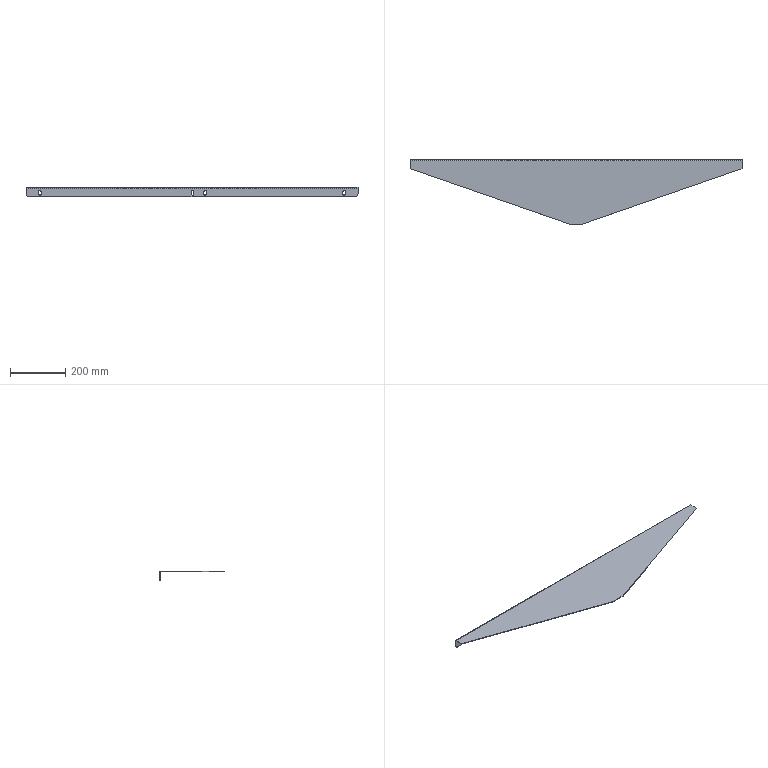Part | SolidWorks | features MirrorStock 1 | 1 solid | 38 faces | box 1200 x 232 x 34 mm | volume 400369 mm3 | plane 22 | cylinder 16 | commonest cylinder face diameters 9 x12 20 x2 2 x1 6 x1
STEP:
#1=CARTESIAN_POINT('',(45.5,0.,-26.));
#2=VERTEX_POINT('',#1);
#3=CARTESIAN_POINT('',(50.,0.,-30.5));
#4=VERTEX_POINT('',#3);
#5=CARTESIAN_POINT('',(50.,0.,-26.));
#6=DIRECTION('',(0.,-1.,0.));
#7=DIRECTION('',(0.,0.,-1.));
#8=AXIS2_PLACEMENT_3D('',#5,#6,#7);
#9=CIRCLE('',#8,4.5);
#10=EDGE_CURVE('',#2,#4,#9,.T.);
#11=ORIENTED_EDGE('',*,*,#10,.T.);
#12=CARTESIAN_POINT('',(50.,2.,-30.5));
#13=VERTEX_POINT('',#12);
#14=CARTESIAN_POINT('',(50.,-8.,-30.5));
#15=DIRECTION('',(0.,1.,0.));
#16=VECTOR('',#15,1000.);
#17=LINE('',#14,#16);
#18=EDGE_CURVE('',#4,#13,#17,.T.);
#19=ORIENTED_EDGE('',*,*,#18,.T.);
#20=CARTESIAN_POINT('',(45.5,2.,-26.));
#21=VERTEX_POINT('',#20);
#22=CARTESIAN_POINT('',(50.,2.,-26.));
#23=DIRECTION('',(0.,-1.,0.));
#24=DIRECTION('',(0.,0.,-1.));
#25=AXIS2_PLACEMENT_3D('',#22,#23,#24);
#26=CIRCLE('',#25,4.5);
#27=EDGE_CURVE('',#21,#13,#26,.T.);
#28=ORIENTED_EDGE('',*,*,#27,.F.);
#29=CARTESIAN_POINT('',(45.5,-8.,-26.));
#30=DIRECTION('',(0.,1.,0.));
#31=VECTOR('',#30,1000.);
#32=LINE('',#29,#31);
#33=EDGE_CURVE('',#2,#21,#32,.T.);
#34=ORIENTED_EDGE('',*,*,#33,.F.);
#35=EDGE_LOOP('',(#11,#19,#28,#34));
#36=FACE_OUTER_BOUND('',#35,.T.);
#37=CARTESIAN_POINT('',(50.,-8.,-26.));
#38=DIRECTION('',(0.,1.,0.));
#39=DIRECTION('',(0.,0.,-1.));
#40=AXIS2_PLACEMENT_3D('',#37,#38,#39);
#41=CYLINDRICAL_SURFACE('',#40,4.5);
#42=ADVANCED_FACE('',(#36),#41,.F.);
#43=CARTESIAN_POINT('',(1145.5,0.,-26.));
#44=VERTEX_POINT('',#43);
#45=CARTESIAN_POINT('',(1150.,0.,-30.5));
#46=VERTEX_POINT('',#45);
#47=CARTESIAN_POINT('',(1150.,0.,-26.));
#48=DIRECTION('',(0.,-1.,0.));
#49=DIRECTION('',(0.,0.,-1.));
#50=AXIS2_PLACEMENT_3D('',#47,#48,#49);
#51=CIRCLE('',#50,4.5);
#52=EDGE_CURVE('',#44,#46,#51,.T.);
#53=ORIENTED_EDGE('',*,*,#52,.T.);
#54=CARTESIAN_POINT('',(1150.,2.,-30.5));
#55=VERTEX_POINT('',#54);
#56=CARTESIAN_POINT('',(1150.,-8.,-30.5));
#57=DIRECTION('',(0.,1.,0.));
#58=VECTOR('',#57,1000.);
#59=LINE('',#56,#58);
#60=EDGE_CURVE('',#46,#55,#59,.T.);
#61=ORIENTED_EDGE('',*,*,#60,.T.);
#62=CARTESIAN_POINT('',(1145.5,2.,-26.));
#63=VERTEX_POINT('',#62);
#64=CARTESIAN_POINT('',(1150.,2.,-26.));
#65=DIRECTION('',(0.,-1.,0.));
#66=DIRECTION('',(0.,0.,-1.));
#67=AXIS2_PLACEMENT_3D('',#64,#65,#66);
#68=CIRCLE('',#67,4.5);
#69=EDGE_CURVE('',#63,#55,#68,.T.);
#70=ORIENTED_EDGE('',*,*,#69,.F.);
#71=CARTESIAN_POINT('',(1145.5,-8.,-26.));
#72=DIRECTION('',(0.,1.,0.));
#73=VECTOR('',#72,1000.);
#74=LINE('',#71,#73);
#75=EDGE_CURVE('',#44,#63,#74,.T.);
#76=ORIENTED_EDGE('',*,*,#75,.F.);
#77=EDGE_LOOP('',(#53,#61,#70,#76));
#78=FACE_OUTER_BOUND('',#77,.T.);
#79=CARTESIAN_POINT('',(1150.,-8.,-26.));
#80=DIRECTION('',(0.,1.,0.));
#81=DIRECTION('',(0.,0.,-1.));
#82=AXIS2_PLACEMENT_3D('',#79,#80,#81);
#83=CYLINDRICAL_SURFACE('',#82,4.5);
#84=ADVANCED_FACE('',(#78),#83,.F.);
#85=CARTESIAN_POINT('',(598.,0.,-26.));
#86=VERTEX_POINT('',#85);
#87=CARTESIAN_POINT('',(602.5,0.,-30.5));
#88=VERTEX_POINT('',#87);
#89=CARTESIAN_POINT('',(602.5,0.,-26.));
#90=DIRECTION('',(0.,-1.,0.));
#91=DIRECTION('',(0.,0.,-1.));
#92=AXIS2_PLACEMENT_3D('',#89,#90,#91);
#93=CIRCLE('',#92,4.5);
#94=EDGE_CURVE('',#86,#88,#93,.T.);
#95=ORIENTED_EDGE('',*,*,#94,.T.);
#96=CARTESIAN_POINT('',(602.5,2.,-30.5));
#97=VERTEX_POINT('',#96);
#98=CARTESIAN_POINT('',(602.5,-8.,-30.5));
#99=DIRECTION('',(0.,1.,0.));
#100=VECTOR('',#99,1000.);
#101=LINE('',#98,#100);
#102=EDGE_CURVE('',#88,#97,#101,.T.);
#103=ORIENTED_EDGE('',*,*,#102,.T.);
#104=CARTESIAN_POINT('',(598.,2.,-26.));
#105=VERTEX_POINT('',#104);
#106=CARTESIAN_POINT('',(602.5,2.,-26.));
#107=DIRECTION('',(0.,-1.,0.));
#108=DIRECTION('',(0.,0.,-1.));
#109=AXIS2_PLACEMENT_3D('',#106,#107,#108);
#110=CIRCLE('',#109,4.5);
#111=EDGE_CURVE('',#105,#97,#110,.T.);
#112=ORIENTED_EDGE('',*,*,#111,.F.);
#113=CARTESIAN_POINT('',(598.,-8.,-26.));
#114=DIRECTION('',(0.,1.,0.));
#115=VECTOR('',#114,1000.);
#116=LINE('',#113,#115);
#117=EDGE_CURVE('',#86,#105,#116,.T.);
#118=ORIENTED_EDGE('',*,*,#117,.F.);
#119=EDGE_LOOP('',(#95,#103,#112,#118));
#120=FACE_OUTER_BOUND('',#119,.T.);
#121=CARTESIAN_POINT('',(602.5,-8.,-26.));
#122=DIRECTION('',(0.,1.,0.));
#123=DIRECTION('',(0.,0.,-1.));
#124=AXIS2_PLACEMENT_3D('',#121,#122,#123);
#125=CYLINDRICAL_SURFACE('',#124,4.5);
#126=ADVANCED_FACE('',(#120),#125,.F.);
#127=CARTESIAN_POINT('',(643.,0.,-26.));
#128=VERTEX_POINT('',#127);
#129=CARTESIAN_POINT('',(647.5,0.,-30.5));
#130=VERTEX_POINT('',#129);
#131=CARTESIAN_POINT('',(647.5,0.,-26.));
#132=DIRECTION('',(0.,-1.,0.));
#133=DIRECTION('',(0.,0.,-1.));
#134=AXIS2_PLACEMENT_3D('',#131,#132,#133);
#135=CIRCLE('',#134,4.5);
#136=EDGE_CURVE('',#128,#130,#135,.T.);
#137=ORIENTED_EDGE('',*,*,#136,.T.);
#138=CARTESIAN_POINT('',(647.5,2.,-30.5));
#139=VERTEX_POINT('',#138);
#140=CARTESIAN_POINT('',(647.5,-8.,-30.5));
#141=DIRECTION('',(0.,1.,0.));
#142=VECTOR('',#141,1000.);
#143=LINE('',#140,#142);
#144=EDGE_CURVE('',#130,#139,#143,.T.);
#145=ORIENTED_EDGE('',*,*,#144,.T.);
#146=CARTESIAN_POINT('',(643.,2.,-26.));
#147=VERTEX_POINT('',#146);
#148=CARTESIAN_POINT('',(647.5,2.,-26.));
#149=DIRECTION('',(0.,-1.,0.));
#150=DIRECTION('',(0.,0.,1.));
#151=AXIS2_PLACEMENT_3D('',#148,#149,#150);
#152=CIRCLE('',#151,4.5);
#153=EDGE_CURVE('',#147,#139,#152,.T.);
#154=ORIENTED_EDGE('',*,*,#153,.F.);
#155=CARTESIAN_POINT('',(643.,-8.,-26.));
#156=DIRECTION('',(0.,1.,0.));
#157=VECTOR('',#156,1000.);
#158=LINE('',#155,#157);
#159=EDGE_CURVE('',#128,#147,#158,.T.);
#160=ORIENTED_EDGE('',*,*,#159,.F.);
#161=EDGE_LOOP('',(#137,#145,#154,#160));
#162=FACE_OUTER_BOUND('',#161,.T.);
#163=CARTESIAN_POINT('',(647.5,-8.,-26.));
#164=DIRECTION('',(0.,1.,0.));
#165=DIRECTION('',(0.,0.,-1.));
#166=AXIS2_PLACEMENT_3D('',#163,#164,#165);
#167=CYLINDRICAL_SURFACE('',#166,4.5);
#168=ADVANCED_FACE('',(#162),#167,.F.);
#169=CARTESIAN_POINT('',(0.,-1.,-4.));
#170=VERTEX_POINT('',#169);
#171=CARTESIAN_POINT('',(0.,-30.,-4.));
#172=VERTEX_POINT('',#171);
#173=CARTESIAN_POINT('',(0.,0.,-4.));
#174=DIRECTION('',(0.,-1.,0.));
#175=VECTOR('',#174,1000.);
#176=LINE('',#173,#175);
#177=EDGE_CURVE('',#170,#172,#176,.T.);
#178=ORIENTED_EDGE('',*,*,#177,.T.);
#179=CARTESIAN_POINT('',(0.,-30.,-2.));
#180=VERTEX_POINT('',#179);
#181=CARTESIAN_POINT('',(0.,-30.,-2.));
#182=DIRECTION('',(0.,0.,-1.));
#183=VECTOR('',#182,1000.);
#184=LINE('',#181,#183);
#185=EDGE_CURVE('',#180,#172,#184,.T.);
#186=ORIENTED_EDGE('',*,*,#185,.F.);
#187=CARTESIAN_POINT('',(0.,-1.,-2.));
#188=VERTEX_POINT('',#187);
#189=CARTESIAN_POINT('',(0.,0.,-2.));
#190=DIRECTION('',(0.,-1.,0.));
#191=VECTOR('',#190,1000.);
#192=LINE('',#189,#191);
#193=EDGE_CURVE('',#188,#180,#192,.T.);
#194=ORIENTED_EDGE('',*,*,#193,.F.);
#195=CARTESIAN_POINT('',(0.,-1.,-4.));
#196=DIRECTION('',(0.,0.,1.));
#197=VECTOR('',#196,1000.);
#198=LINE('',#195,#197);
#199=EDGE_CURVE('',#170,#188,#198,.T.);
#200=ORIENTED_EDGE('',*,*,#199,.F.);
#201=EDGE_LOOP('',(#178,#186,#194,#200));
#202=FACE_OUTER_BOUND('',#201,.T.);
#203=CARTESIAN_POINT('',(0.,0.,-2.));
#204=DIRECTION('',(-1.,0.,0.));
#205=DIRECTION('',(0.,-1.,0.));
#206=AXIS2_PLACEMENT_3D('',#203,#204,#205);
#207=PLANE('',#206);
#208=ADVANCED_FACE('',(#202),#207,.T.);
#209=ORIENTED_EDGE('',*,*,#193,.T.);
#210=CARTESIAN_POINT('',(575.,-230.,-2.));
#211=VERTEX_POINT('',#210);
#212=CARTESIAN_POINT('',(0.,-30.,-2.));
#213=DIRECTION('',(0.9445,-0.3285,0.));
#214=VECTOR('',#213,1000.);
#215=LINE('',#212,#214);
#216=EDGE_CURVE('',#180,#211,#215,.T.);
#217=ORIENTED_EDGE('',*,*,#216,.T.);
#218=CARTESIAN_POINT('',(625.,-230.,-2.));
#219=VERTEX_POINT('',#218);
#220=CARTESIAN_POINT('',(625.,-230.,-2.));
#221=DIRECTION('',(1.,0.,0.));
#222=VECTOR('',#221,1000.);
#223=LINE('',#220,#222);
#224=EDGE_CURVE('',#211,#219,#223,.T.);
#225=ORIENTED_EDGE('',*,*,#224,.T.);
#226=CARTESIAN_POINT('',(1200.,-30.,-2.));
#227=VERTEX_POINT('',#226);
#228=CARTESIAN_POINT('',(1200.,-30.,-2.));
#229=DIRECTION('',(0.9445,0.3285,0.));
#230=VECTOR('',#229,1000.);
#231=LINE('',#228,#230);
#232=EDGE_CURVE('',#219,#227,#231,.T.);
#233=ORIENTED_EDGE('',*,*,#232,.T.);
#234=CARTESIAN_POINT('',(1200.,-1.,-2.));
#235=VERTEX_POINT('',#234);
#236=CARTESIAN_POINT('',(1200.,0.,-2.));
#237=DIRECTION('',(0.,1.,0.));
#238=VECTOR('',#237,1000.);
#239=LINE('',#236,#238);
#240=EDGE_CURVE('',#227,#235,#239,.T.);
#241=ORIENTED_EDGE('',*,*,#240,.T.);
#242=CARTESIAN_POINT('',(0.,-1.,-2.));
#243=DIRECTION('',(1.,0.,0.));
#244=VECTOR('',#243,1000.);
#245=LINE('',#242,#244);
#246=EDGE_CURVE('',#188,#235,#245,.T.);
#247=ORIENTED_EDGE('',*,*,#246,.F.);
#248=EDGE_LOOP('',(#209,#217,#225,#233,#241,#247));
#249=FACE_OUTER_BOUND('',#248,.T.);
#250=CARTESIAN_POINT('',(0.,0.,-2.));
#251=DIRECTION('',(0.,0.,1.));
#252=DIRECTION('',(-1.,0.,0.));
#253=AXIS2_PLACEMENT_3D('',#250,#251,#252);
#254=PLANE('',#253);
#255=ADVANCED_FACE('',(#249),#254,.T.);
#256=CARTESIAN_POINT('',(1200.,-1.,-4.));
#257=VERTEX_POINT('',#256);
#258=CARTESIAN_POINT('',(0.,-1.,-4.));
#259=DIRECTION('',(1.,0.,0.));
#260=VECTOR('',#259,1000.);
#261=LINE('',#258,#260);
#262=EDGE_CURVE('',#170,#257,#261,.T.);
#263=ORIENTED_EDGE('',*,*,#262,.T.);
#264=CARTESIAN_POINT('',(1200.,-30.,-4.));
#265=VERTEX_POINT('',#264);
#266=CARTESIAN_POINT('',(1200.,0.,-4.));
#267=DIRECTION('',(0.,1.,0.));
#268=VECTOR('',#267,1000.);
#269=LINE('',#266,#268);
#270=EDGE_CURVE('',#265,#257,#269,.T.);
#271=ORIENTED_EDGE('',*,*,#270,.F.);
#272=CARTESIAN_POINT('',(625.,-230.,-4.));
#273=VERTEX_POINT('',#272);
#274=CARTESIAN_POINT('',(1200.,-30.,-4.));
#275=DIRECTION('',(0.9445,0.3285,0.));
#276=VECTOR('',#275,1000.);
#277=LINE('',#274,#276);
#278=EDGE_CURVE('',#273,#265,#277,.T.);
#279=ORIENTED_EDGE('',*,*,#278,.F.);
#280=CARTESIAN_POINT('',(575.,-230.,-4.));
#281=VERTEX_POINT('',#280);
#282=CARTESIAN_POINT('',(625.,-230.,-4.));
#283=DIRECTION('',(1.,0.,0.));
#284=VECTOR('',#283,1000.);
#285=LINE('',#282,#284);
#286=EDGE_CURVE('',#281,#273,#285,.T.);
#287=ORIENTED_EDGE('',*,*,#286,.F.);
#288=CARTESIAN_POINT('',(0.,-30.,-4.));
#289=DIRECTION('',(0.9445,-0.3285,0.));
#290=VECTOR('',#289,1000.);
#291=LINE('',#288,#290);
#292=EDGE_CURVE('',#172,#281,#291,.T.);
#293=ORIENTED_EDGE('',*,*,#292,.F.);
#294=ORIENTED_EDGE('',*,*,#177,.F.);
#295=EDGE_LOOP('',(#263,#271,#279,#287,#293,#294));
#296=FACE_OUTER_BOUND('',#295,.T.);
#297=CARTESIAN_POINT('',(0.,0.,-4.));
#298=DIRECTION('',(0.,0.,1.));
#299=DIRECTION('',(-1.,0.,0.));
#300=AXIS2_PLACEMENT_3D('',#297,#298,#299);
#301=PLANE('',#300);
#302=ADVANCED_FACE('',(#296),#301,.F.);
#303=CARTESIAN_POINT('',(1200.,-1.,-4.));
#304=DIRECTION('',(0.,0.,1.));
#305=VECTOR('',#304,1000.);
#306=LINE('',#303,#305);
#307=EDGE_CURVE('',#257,#235,#306,.T.);
#308=ORIENTED_EDGE('',*,*,#307,.T.);
#309=ORIENTED_EDGE('',*,*,#240,.F.);
#310=CARTESIAN_POINT('',(1200.,-30.,-2.));
#311=DIRECTION('',(0.,0.,-1.));
#312=VECTOR('',#311,1000.);
#313=LINE('',#310,#312);
#314=EDGE_CURVE('',#227,#265,#313,.T.);
#315=ORIENTED_EDGE('',*,*,#314,.T.);
#316=ORIENTED_EDGE('',*,*,#270,.T.);
#317=EDGE_LOOP('',(#308,#309,#315,#316));
#318=FACE_OUTER_BOUND('',#317,.T.);
#319=CARTESIAN_POINT('',(1200.,0.,-2.));
#320=DIRECTION('',(1.,0.,0.));
#321=DIRECTION('',(0.,0.,1.));
#322=AXIS2_PLACEMENT_3D('',#319,#320,#321);
#323=PLANE('',#322);
#324=ADVANCED_FACE('',(#318),#323,.T.);
#325=ORIENTED_EDGE('',*,*,#278,.T.);
#326=ORIENTED_EDGE('',*,*,#314,.F.);
#327=ORIENTED_EDGE('',*,*,#232,.F.);
#328=CARTESIAN_POINT('',(625.,-230.,-2.));
#329=DIRECTION('',(0.,0.,-1.));
#330=VECTOR('',#329,1000.);
#331=LINE('',#328,#330);
#332=EDGE_CURVE('',#219,#273,#331,.T.);
#333=ORIENTED_EDGE('',*,*,#332,.T.);
#334=EDGE_LOOP('',(#325,#326,#327,#333));
#335=FACE_OUTER_BOUND('',#334,.T.);
#336=CARTESIAN_POINT('',(1200.,-30.,-2.));
#337=DIRECTION('',(0.3285,-0.9445,0.));
#338=DIRECTION('',(0.9445,0.3285,0.));
#339=AXIS2_PLACEMENT_3D('',#336,#337,#338);
#340=PLANE('',#339);
#341=ADVANCED_FACE('',(#335),#340,.T.);
#342=ORIENTED_EDGE('',*,*,#286,.T.);
#343=ORIENTED_EDGE('',*,*,#332,.F.);
#344=ORIENTED_EDGE('',*,*,#224,.F.);
#345=CARTESIAN_POINT('',(575.,-230.,-2.));
#346=DIRECTION('',(0.,0.,-1.));
#347=VECTOR('',#346,1000.);
#348=LINE('',#345,#347);
#349=EDGE_CURVE('',#211,#281,#348,.T.);
#350=ORIENTED_EDGE('',*,*,#349,.T.);
#351=EDGE_LOOP('',(#342,#343,#344,#350));
#352=FACE_OUTER_BOUND('',#351,.T.);
#353=CARTESIAN_POINT('',(625.,-230.,-2.));
#354=DIRECTION('',(0.,-1.,0.));
#355=DIRECTION('',(0.,0.,1.));
#356=AXIS2_PLACEMENT_3D('',#353,#354,#355);
#357=PLANE('',#356);
#358=ADVANCED_FACE('',(#352),#357,.T.);
#359=ORIENTED_EDGE('',*,*,#292,.T.);
#360=ORIENTED_EDGE('',*,*,#349,.F.);
#361=ORIENTED_EDGE('',*,*,#216,.F.);
#362=ORIENTED_EDGE('',*,*,#185,.T.);
#363=EDGE_LOOP('',(#359,#360,#361,#362));
#364=FACE_OUTER_BOUND('',#363,.T.);
#365=CARTESIAN_POINT('',(0.,-30.,-2.));
#366=DIRECTION('',(-0.3285,-0.9445,0.));
#367=DIRECTION('',(0.9445,-0.3285,0.));
#368=AXIS2_PLACEMENT_3D('',#365,#366,#367);
#369=PLANE('',#368);
#370=ADVANCED_FACE('',(#364),#369,.T.);
#371=CARTESIAN_POINT('',(1200.,0.,-5.));
#372=VERTEX_POINT('',#371);
#373=CARTESIAN_POINT('',(1200.,2.,-5.));
#374=VERTEX_POINT('',#373);
#375=CARTESIAN_POINT('',(1200.,0.,-5.));
#376=DIRECTION('',(0.,1.,0.));
#377=VECTOR('',#376,1000.);
#378=LINE('',#375,#377);
#379=EDGE_CURVE('',#372,#374,#378,.T.);
#380=ORIENTED_EDGE('',*,*,#379,.T.);
#381=CARTESIAN_POINT('',(1200.,-1.,-5.));
#382=DIRECTION('',(-1.,0.,0.));
#383=DIRECTION('',(0.,0.,-1.));
#384=AXIS2_PLACEMENT_3D('',#381,#382,#383);
#385=CIRCLE('',#384,3.);
#386=EDGE_CURVE('',#235,#374,#385,.T.);
#387=ORIENTED_EDGE('',*,*,#386,.F.);
#388=ORIENTED_EDGE('',*,*,#307,.F.);
#389=CARTESIAN_POINT('',(1200.,-1.,-5.));
#390=DIRECTION('',(-1.,0.,0.));
#391=DIRECTION('',(0.,0.,-1.));
#392=AXIS2_PLACEMENT_3D('',#389,#390,#391);
#393=CIRCLE('',#392,1.);
#394=EDGE_CURVE('',#257,#372,#393,.T.);
#395=ORIENTED_EDGE('',*,*,#394,.T.);
#396=EDGE_LOOP('',(#380,#387,#388,#395));
#397=FACE_OUTER_BOUND('',#396,.T.);
#398=CARTESIAN_POINT('',(1200.,-1.,-5.));
#399=DIRECTION('',(1.,0.,0.));
#400=DIRECTION('',(0.,0.,1.));
#401=AXIS2_PLACEMENT_3D('',#398,#399,#400);
#402=PLANE('',#401);
#403=ADVANCED_FACE('',(#397),#402,.T.);
#404=CARTESIAN_POINT('',(0.,0.,-5.));
#405=VERTEX_POINT('',#404);
#406=CARTESIAN_POINT('',(0.,-1.,-5.));
#407=DIRECTION('',(1.,0.,0.));
#408=DIRECTION('',(0.,0.,-1.));
#409=AXIS2_PLACEMENT_3D('',#406,#407,#408);
#410=CIRCLE('',#409,1.);
#411=EDGE_CURVE('',#405,#170,#410,.T.);
#412=ORIENTED_EDGE('',*,*,#411,.T.);
#413=ORIENTED_EDGE('',*,*,#199,.T.);
#414=CARTESIAN_POINT('',(0.,2.,-5.));
#415=VERTEX_POINT('',#414);
#416=CARTESIAN_POINT('',(0.,-1.,-5.));
#417=DIRECTION('',(1.,0.,0.));
#418=DIRECTION('',(0.,0.,-1.));
#419=AXIS2_PLACEMENT_3D('',#416,#417,#418);
#420=CIRCLE('',#419,3.);
#421=EDGE_CURVE('',#415,#188,#420,.T.);
#422=ORIENTED_EDGE('',*,*,#421,.F.);
#423=CARTESIAN_POINT('',(0.,0.,-5.));
#424=DIRECTION('',(0.,1.,0.));
#425=VECTOR('',#424,1000.);
#426=LINE('',#423,#425);
#427=EDGE_CURVE('',#405,#415,#426,.T.);
#428=ORIENTED_EDGE('',*,*,#427,.F.);
#429=EDGE_LOOP('',(#412,#413,#422,#428));
#430=FACE_OUTER_BOUND('',#429,.T.);
#431=CARTESIAN_POINT('',(0.,-1.,-5.));
#432=DIRECTION('',(1.,0.,0.));
#433=DIRECTION('',(0.,0.,1.));
#434=AXIS2_PLACEMENT_3D('',#431,#432,#433);
#435=PLANE('',#434);
#436=ADVANCED_FACE('',(#430),#435,.F.);
#437=ORIENTED_EDGE('',*,*,#246,.T.);
#438=ORIENTED_EDGE('',*,*,#386,.T.);
#439=CARTESIAN_POINT('',(0.,2.,-5.));
#440=DIRECTION('',(-1.,0.,0.));
#441=VECTOR('',#440,1000.);
#442=LINE('',#439,#441);
#443=EDGE_CURVE('',#374,#415,#442,.T.);
#444=ORIENTED_EDGE('',*,*,#443,.T.);
#445=ORIENTED_EDGE('',*,*,#421,.T.);
#446=EDGE_LOOP('',(#437,#438,#444,#445));
#447=FACE_OUTER_BOUND('',#446,.T.);
#448=CARTESIAN_POINT('',(0.,-1.,-5.));
#449=DIRECTION('',(-1.,0.,0.));
#450=DIRECTION('',(0.,1.,0.));
#451=AXIS2_PLACEMENT_3D('',#448,#449,#450);
#452=CYLINDRICAL_SURFACE('',#451,3.);
#453=ADVANCED_FACE('',(#447),#452,.T.);
#454=ORIENTED_EDGE('',*,*,#262,.F.);
#455=ORIENTED_EDGE('',*,*,#411,.F.);
#456=CARTESIAN_POINT('',(1200.,0.,-5.));
#457=DIRECTION('',(-1.,0.,0.));
#458=VECTOR('',#457,1000.);
#459=LINE('',#456,#458);
#460=EDGE_CURVE('',#372,#405,#459,.T.);
#461=ORIENTED_EDGE('',*,*,#460,.F.);
#462=ORIENTED_EDGE('',*,*,#394,.F.);
#463=EDGE_LOOP('',(#454,#455,#461,#462));
#464=FACE_OUTER_BOUND('',#463,.T.);
#465=CARTESIAN_POINT('',(0.,-1.,-5.));
#466=DIRECTION('',(-1.,0.,0.));
#467=DIRECTION('',(0.,1.,0.));
#468=AXIS2_PLACEMENT_3D('',#465,#466,#467);
#469=CYLINDRICAL_SURFACE('',#468,1.);
#470=ADVANCED_FACE('',(#464),#469,.F.);
#471=CARTESIAN_POINT('',(1200.,2.,-26.));
#472=VERTEX_POINT('',#471);
#473=CARTESIAN_POINT('',(1200.,2.,-36.));
#474=DIRECTION('',(0.,0.,-1.));
#475=VECTOR('',#474,1000.);
#476=LINE('',#473,#475);
#477=EDGE_CURVE('',#374,#472,#476,.T.);
#478=ORIENTED_EDGE('',*,*,#477,.F.);
#479=ORIENTED_EDGE('',*,*,#379,.F.);
#480=CARTESIAN_POINT('',(1200.,0.,-26.));
#481=VERTEX_POINT('',#480);
#482=CARTESIAN_POINT('',(1200.,0.,-36.));
#483=DIRECTION('',(0.,0.,-1.));
#484=VECTOR('',#483,1000.);
#485=LINE('',#482,#484);
#486=EDGE_CURVE('',#372,#481,#485,.T.);
#487=ORIENTED_EDGE('',*,*,#486,.T.);
#488=CARTESIAN_POINT('',(1200.,2.,-26.));
#489=DIRECTION('',(0.,-1.,0.));
#490=VECTOR('',#489,1000.);
#491=LINE('',#488,#490);
#492=EDGE_CURVE('',#472,#481,#491,.T.);
#493=ORIENTED_EDGE('',*,*,#492,.F.);
#494=EDGE_LOOP('',(#478,#479,#487,#493));
#495=FACE_OUTER_BOUND('',#494,.T.);
#496=CARTESIAN_POINT('',(1200.,2.,-36.));
#497=DIRECTION('',(1.,0.,0.));
#498=DIRECTION('',(0.,0.,1.));
#499=AXIS2_PLACEMENT_3D('',#496,#497,#498);
#500=PLANE('',#499);
#501=ADVANCED_FACE('',(#495),#500,.T.);
#502=CARTESIAN_POINT('',(0.,0.,-26.));
#503=VERTEX_POINT('',#502);
#504=CARTESIAN_POINT('',(0.,0.,-4.));
#505=DIRECTION('',(0.,0.,1.));
#506=VECTOR('',#505,1000.);
#507=LINE('',#504,#506);
#508=EDGE_CURVE('',#503,#405,#507,.T.);
#509=ORIENTED_EDGE('',*,*,#508,.T.);
#510=ORIENTED_EDGE('',*,*,#427,.T.);
#511=CARTESIAN_POINT('',(0.,2.,-26.));
#512=VERTEX_POINT('',#511);
#513=CARTESIAN_POINT('',(0.,2.,-4.));
#514=DIRECTION('',(0.,0.,1.));
#515=VECTOR('',#514,1000.);
#516=LINE('',#513,#515);
#517=EDGE_CURVE('',#512,#415,#516,.T.);
#518=ORIENTED_EDGE('',*,*,#517,.F.);
#519=CARTESIAN_POINT('',(0.,2.,-26.));
#520=DIRECTION('',(0.,1.,0.));
#521=VECTOR('',#520,1000.);
#522=LINE('',#519,#521);
#523=EDGE_CURVE('',#503,#512,#522,.T.);
#524=ORIENTED_EDGE('',*,*,#523,.F.);
#525=EDGE_LOOP('',(#509,#510,#518,#524));
#526=FACE_OUTER_BOUND('',#525,.T.);
#527=CARTESIAN_POINT('',(0.,2.,-4.));
#528=DIRECTION('',(-1.,0.,0.));
#529=DIRECTION('',(0.,0.,-1.));
#530=AXIS2_PLACEMENT_3D('',#527,#528,#529);
#531=PLANE('',#530);
#532=ADVANCED_FACE('',(#526),#531,.T.);
#533=CARTESIAN_POINT('',(54.5,2.,-18.));
#534=VERTEX_POINT('',#533);
#535=CARTESIAN_POINT('',(45.5,2.,-18.));
#536=VERTEX_POINT('',#535);
#537=CARTESIAN_POINT('',(50.,2.,-18.));
#538=DIRECTION('',(0.,-1.,0.));
#539=DIRECTION('',(0.,0.,-1.));
#540=AXIS2_PLACEMENT_3D('',#537,#538,#539);
#541=CIRCLE('',#540,4.5);
#542=EDGE_CURVE('',#534,#536,#541,.T.);
#543=ORIENTED_EDGE('',*,*,#542,.T.);
#544=CARTESIAN_POINT('',(45.5,2.,-18.));
#545=DIRECTION('',(0.,0.,-1.));
#546=VECTOR('',#545,1000.);
#547=LINE('',#544,#546);
#548=EDGE_CURVE('',#536,#21,#547,.T.);
#549=ORIENTED_EDGE('',*,*,#548,.T.);
#550=ORIENTED_EDGE('',*,*,#27,.T.);
#551=CARTESIAN_POINT('',(54.5,2.,-26.));
#552=VERTEX_POINT('',#551);
#553=CARTESIAN_POINT('',(50.,2.,-26.));
#554=DIRECTION('',(0.,-1.,0.));
#555=DIRECTION('',(0.,0.,-1.));
#556=AXIS2_PLACEMENT_3D('',#553,#554,#555);
#557=CIRCLE('',#556,4.5);
#558=EDGE_CURVE('',#13,#552,#557,.T.);
#559=ORIENTED_EDGE('',*,*,#558,.T.);
#560=CARTESIAN_POINT('',(54.5,2.,-18.));
#561=DIRECTION('',(0.,0.,1.));
#562=VECTOR('',#561,1000.);
#563=LINE('',#560,#562);
#564=EDGE_CURVE('',#552,#534,#563,.T.);
#565=ORIENTED_EDGE('',*,*,#564,.T.);
#566=EDGE_LOOP('',(#543,#549,#550,#559,#565));
#567=FACE_BOUND('',#566,.T.);
#568=CARTESIAN_POINT('',(1154.5,2.,-18.));
#569=VERTEX_POINT('',#568);
#570=CARTESIAN_POINT('',(1145.5,2.,-18.));
#571=VERTEX_POINT('',#570);
#572=CARTESIAN_POINT('',(1150.,2.,-18.));
#573=DIRECTION('',(0.,-1.,0.));
#574=DIRECTION('',(0.,0.,-1.));
#575=AXIS2_PLACEMENT_3D('',#572,#573,#574);
#576=CIRCLE('',#575,4.5);
#577=EDGE_CURVE('',#569,#571,#576,.T.);
#578=ORIENTED_EDGE('',*,*,#577,.T.);
#579=CARTESIAN_POINT('',(1145.5,2.,-18.));
#580=DIRECTION('',(0.,0.,-1.));
#581=VECTOR('',#580,1000.);
#582=LINE('',#579,#581);
#583=EDGE_CURVE('',#571,#63,#582,.T.);
#584=ORIENTED_EDGE('',*,*,#583,.T.);
#585=ORIENTED_EDGE('',*,*,#69,.T.);
#586=CARTESIAN_POINT('',(1154.5,2.,-26.));
#587=VERTEX_POINT('',#586);
#588=CARTESIAN_POINT('',(1150.,2.,-26.));
#589=DIRECTION('',(0.,-1.,0.));
#590=DIRECTION('',(0.,0.,-1.));
#591=AXIS2_PLACEMENT_3D('',#588,#589,#590);
#592=CIRCLE('',#591,4.5);
#593=EDGE_CURVE('',#55,#587,#592,.T.);
#594=ORIENTED_EDGE('',*,*,#593,.T.);
#595=CARTESIAN_POINT('',(1154.5,2.,-18.));
#596=DIRECTION('',(0.,0.,1.));
#597=VECTOR('',#596,1000.);
#598=LINE('',#595,#597);
#599=EDGE_CURVE('',#587,#569,#598,.T.);
#600=ORIENTED_EDGE('',*,*,#599,.T.);
#601=EDGE_LOOP('',(#578,#584,#585,#594,#600));
#602=FACE_BOUND('',#601,.T.);
#603=CARTESIAN_POINT('',(607.,2.,-18.));
#604=VERTEX_POINT('',#603);
#605=CARTESIAN_POINT('',(598.,2.,-18.));
#606=VERTEX_POINT('',#605);
#607=CARTESIAN_POINT('',(602.5,2.,-18.));
#608=DIRECTION('',(0.,-1.,0.));
#609=DIRECTION('',(0.,0.,-1.));
#610=AXIS2_PLACEMENT_3D('',#607,#608,#609);
#611=CIRCLE('',#610,4.5);
#612=EDGE_CURVE('',#604,#606,#611,.T.);
#613=ORIENTED_EDGE('',*,*,#612,.T.);
#614=CARTESIAN_POINT('',(598.,2.,-18.));
#615=DIRECTION('',(0.,0.,-1.));
#616=VECTOR('',#615,1000.);
#617=LINE('',#614,#616);
#618=EDGE_CURVE('',#606,#105,#617,.T.);
#619=ORIENTED_EDGE('',*,*,#618,.T.);
#620=ORIENTED_EDGE('',*,*,#111,.T.);
#621=CARTESIAN_POINT('',(607.,2.,-26.));
#622=VERTEX_POINT('',#621);
#623=CARTESIAN_POINT('',(602.5,2.,-26.));
#624=DIRECTION('',(0.,-1.,0.));
#625=DIRECTION('',(0.,0.,-1.));
#626=AXIS2_PLACEMENT_3D('',#623,#624,#625);
#627=CIRCLE('',#626,4.5);
#628=EDGE_CURVE('',#97,#622,#627,.T.);
#629=ORIENTED_EDGE('',*,*,#628,.T.);
#630=CARTESIAN_POINT('',(607.,2.,-18.));
#631=DIRECTION('',(0.,0.,1.));
#632=VECTOR('',#631,1000.);
#633=LINE('',#630,#632);
#634=EDGE_CURVE('',#622,#604,#633,.T.);
#635=ORIENTED_EDGE('',*,*,#634,.T.);
#636=EDGE_LOOP('',(#613,#619,#620,#629,#635));
#637=FACE_BOUND('',#636,.T.);
#638=CARTESIAN_POINT('',(652.,2.,-18.));
#639=VERTEX_POINT('',#638);
#640=CARTESIAN_POINT('',(643.,2.,-18.));
#641=VERTEX_POINT('',#640);
#642=CARTESIAN_POINT('',(647.5,2.,-18.));
#643=DIRECTION('',(0.,-1.,0.));
#644=DIRECTION('',(0.,0.,1.));
#645=AXIS2_PLACEMENT_3D('',#642,#643,#644);
#646=CIRCLE('',#645,4.5);
#647=EDGE_CURVE('',#639,#641,#646,.T.);
#648=ORIENTED_EDGE('',*,*,#647,.T.);
#649=CARTESIAN_POINT('',(643.,2.,-18.));
#650=DIRECTION('',(0.,0.,-1.));
#651=VECTOR('',#650,1000.);
#652=LINE('',#649,#651);
#653=EDGE_CURVE('',#641,#147,#652,.T.);
#654=ORIENTED_EDGE('',*,*,#653,.T.);
#655=ORIENTED_EDGE('',*,*,#153,.T.);
#656=CARTESIAN_POINT('',(652.,2.,-26.));
#657=VERTEX_POINT('',#656);
#658=CARTESIAN_POINT('',(647.5,2.,-26.));
#659=DIRECTION('',(0.,-1.,0.));
#660=DIRECTION('',(0.,0.,1.));
#661=AXIS2_PLACEMENT_3D('',#658,#659,#660);
#662=CIRCLE('',#661,4.5);
#663=EDGE_CURVE('',#139,#657,#662,.T.);
#664=ORIENTED_EDGE('',*,*,#663,.T.);
#665=CARTESIAN_POINT('',(652.,2.,-18.));
#666=DIRECTION('',(0.,0.,1.));
#667=VECTOR('',#666,1000.);
#668=LINE('',#665,#667);
#669=EDGE_CURVE('',#657,#639,#668,.T.);
#670=ORIENTED_EDGE('',*,*,#669,.T.);
#671=EDGE_LOOP('',(#648,#654,#655,#664,#670));
#672=FACE_BOUND('',#671,.T.);
#673=CARTESIAN_POINT('',(1190.,2.,-36.));
#674=VERTEX_POINT('',#673);
#675=CARTESIAN_POINT('',(10.,2.,-36.));
#676=VERTEX_POINT('',#675);
#677=CARTESIAN_POINT('',(0.,2.,-36.));
#678=DIRECTION('',(-1.,0.,0.));
#679=VECTOR('',#678,1000.);
#680=LINE('',#677,#679);
#681=EDGE_CURVE('',#674,#676,#680,.T.);
#682=ORIENTED_EDGE('',*,*,#681,.T.);
#683=CARTESIAN_POINT('',(10.,2.,-26.));
#684=DIRECTION('',(0.,-1.,0.));
#685=DIRECTION('',(0.,0.,-1.));
#686=AXIS2_PLACEMENT_3D('',#683,#684,#685);
#687=CIRCLE('',#686,10.);
#688=EDGE_CURVE('',#512,#676,#687,.T.);
#689=ORIENTED_EDGE('',*,*,#688,.F.);
#690=ORIENTED_EDGE('',*,*,#517,.T.);
#691=ORIENTED_EDGE('',*,*,#443,.F.);
#692=ORIENTED_EDGE('',*,*,#477,.T.);
#693=CARTESIAN_POINT('',(1190.,2.,-26.));
#694=DIRECTION('',(0.,-1.,0.));
#695=DIRECTION('',(0.,0.,-1.));
#696=AXIS2_PLACEMENT_3D('',#693,#694,#695);
#697=CIRCLE('',#696,10.);
#698=EDGE_CURVE('',#674,#472,#697,.T.);
#699=ORIENTED_EDGE('',*,*,#698,.F.);
#700=EDGE_LOOP('',(#682,#689,#690,#691,#692,#699));
#701=FACE_OUTER_BOUND('',#700,.T.);
#702=CARTESIAN_POINT('',(0.,2.,-4.));
#703=DIRECTION('',(0.,1.,0.));
#704=DIRECTION('',(0.,0.,-1.));
#705=AXIS2_PLACEMENT_3D('',#702,#703,#704);
#706=PLANE('',#705);
#707=ADVANCED_FACE('',(#567,#602,#637,#672,#701),#706,.T.);
#708=CARTESIAN_POINT('',(54.5,0.,-26.));
#709=VERTEX_POINT('',#708);
#710=CARTESIAN_POINT('',(54.5,0.,-18.));
#711=VERTEX_POINT('',#710);
#712=CARTESIAN_POINT('',(54.5,0.,-4.));
#713=DIRECTION('',(0.,0.,1.));
#714=VECTOR('',#713,1000.);
#715=LINE('',#712,#714);
#716=EDGE_CURVE('',#709,#711,#715,.T.);
#717=ORIENTED_EDGE('',*,*,#716,.F.);
#718=CARTESIAN_POINT('',(50.,0.,-26.));
#719=DIRECTION('',(0.,-1.,0.));
#720=DIRECTION('',(0.,0.,-1.));
#721=AXIS2_PLACEMENT_3D('',#718,#719,#720);
#722=CIRCLE('',#721,4.5);
#723=EDGE_CURVE('',#4,#709,#722,.T.);
#724=ORIENTED_EDGE('',*,*,#723,.F.);
#725=ORIENTED_EDGE('',*,*,#10,.F.);
#726=CARTESIAN_POINT('',(45.5,0.,-18.));
#727=VERTEX_POINT('',#726);
#728=CARTESIAN_POINT('',(45.5,0.,-4.));
#729=DIRECTION('',(0.,0.,-1.));
#730=VECTOR('',#729,1000.);
#731=LINE('',#728,#730);
#732=EDGE_CURVE('',#727,#2,#731,.T.);
#733=ORIENTED_EDGE('',*,*,#732,.F.);
#734=CARTESIAN_POINT('',(50.,0.,-18.));
#735=DIRECTION('',(0.,-1.,0.));
#736=DIRECTION('',(0.,0.,-1.));
#737=AXIS2_PLACEMENT_3D('',#734,#735,#736);
#738=CIRCLE('',#737,4.5);
#739=EDGE_CURVE('',#711,#727,#738,.T.);
#740=ORIENTED_EDGE('',*,*,#739,.F.);
#741=EDGE_LOOP('',(#717,#724,#725,#733,#740));
#742=FACE_BOUND('',#741,.T.);
#743=CARTESIAN_POINT('',(1154.5,0.,-26.));
#744=VERTEX_POINT('',#743);
#745=CARTESIAN_POINT('',(1154.5,0.,-18.));
#746=VERTEX_POINT('',#745);
#747=CARTESIAN_POINT('',(1154.5,0.,-4.));
#748=DIRECTION('',(0.,0.,1.));
#749=VECTOR('',#748,1000.);
#750=LINE('',#747,#749);
#751=EDGE_CURVE('',#744,#746,#750,.T.);
#752=ORIENTED_EDGE('',*,*,#751,.F.);
#753=CARTESIAN_POINT('',(1150.,0.,-26.));
#754=DIRECTION('',(0.,-1.,0.));
#755=DIRECTION('',(0.,0.,-1.));
#756=AXIS2_PLACEMENT_3D('',#753,#754,#755);
#757=CIRCLE('',#756,4.5);
#758=EDGE_CURVE('',#46,#744,#757,.T.);
#759=ORIENTED_EDGE('',*,*,#758,.F.);
#760=ORIENTED_EDGE('',*,*,#52,.F.);
#761=CARTESIAN_POINT('',(1145.5,0.,-18.));
#762=VERTEX_POINT('',#761);
#763=CARTESIAN_POINT('',(1145.5,0.,-4.));
#764=DIRECTION('',(0.,0.,-1.));
#765=VECTOR('',#764,1000.);
#766=LINE('',#763,#765);
#767=EDGE_CURVE('',#762,#44,#766,.T.);
#768=ORIENTED_EDGE('',*,*,#767,.F.);
#769=CARTESIAN_POINT('',(1150.,0.,-18.));
#770=DIRECTION('',(0.,-1.,0.));
#771=DIRECTION('',(0.,0.,-1.));
#772=AXIS2_PLACEMENT_3D('',#769,#770,#771);
#773=CIRCLE('',#772,4.5);
#774=EDGE_CURVE('',#746,#762,#773,.T.);
#775=ORIENTED_EDGE('',*,*,#774,.F.);
#776=EDGE_LOOP('',(#752,#759,#760,#768,#775));
#777=FACE_BOUND('',#776,.T.);
#778=CARTESIAN_POINT('',(607.,0.,-26.));
#779=VERTEX_POINT('',#778);
#780=CARTESIAN_POINT('',(607.,0.,-18.));
#781=VERTEX_POINT('',#780);
#782=CARTESIAN_POINT('',(607.,0.,-4.));
#783=DIRECTION('',(0.,0.,1.));
#784=VECTOR('',#783,1000.);
#785=LINE('',#782,#784);
#786=EDGE_CURVE('',#779,#781,#785,.T.);
#787=ORIENTED_EDGE('',*,*,#786,.F.);
#788=CARTESIAN_POINT('',(602.5,0.,-26.));
#789=DIRECTION('',(0.,-1.,0.));
#790=DIRECTION('',(0.,0.,-1.));
#791=AXIS2_PLACEMENT_3D('',#788,#789,#790);
#792=CIRCLE('',#791,4.5);
#793=EDGE_CURVE('',#88,#779,#792,.T.);
#794=ORIENTED_EDGE('',*,*,#793,.F.);
#795=ORIENTED_EDGE('',*,*,#94,.F.);
#796=CARTESIAN_POINT('',(598.,0.,-18.));
#797=VERTEX_POINT('',#796);
#798=CARTESIAN_POINT('',(598.,0.,-4.));
#799=DIRECTION('',(0.,0.,-1.));
#800=VECTOR('',#799,1000.);
#801=LINE('',#798,#800);
#802=EDGE_CURVE('',#797,#86,#801,.T.);
#803=ORIENTED_EDGE('',*,*,#802,.F.);
#804=CARTESIAN_POINT('',(602.5,0.,-18.));
#805=DIRECTION('',(0.,-1.,0.));
#806=DIRECTION('',(0.,0.,-1.));
#807=AXIS2_PLACEMENT_3D('',#804,#805,#806);
#808=CIRCLE('',#807,4.5);
#809=EDGE_CURVE('',#781,#797,#808,.T.);
#810=ORIENTED_EDGE('',*,*,#809,.F.);
#811=EDGE_LOOP('',(#787,#794,#795,#803,#810));
#812=FACE_BOUND('',#811,.T.);
#813=CARTESIAN_POINT('',(652.,0.,-26.));
#814=VERTEX_POINT('',#813);
#815=CARTESIAN_POINT('',(652.,0.,-18.));
#816=VERTEX_POINT('',#815);
#817=CARTESIAN_POINT('',(652.,0.,-4.));
#818=DIRECTION('',(0.,0.,1.));
#819=VECTOR('',#818,1000.);
#820=LINE('',#817,#819);
#821=EDGE_CURVE('',#814,#816,#820,.T.);
#822=ORIENTED_EDGE('',*,*,#821,.F.);
#823=CARTESIAN_POINT('',(647.5,0.,-26.));
#824=DIRECTION('',(0.,-1.,0.));
#825=DIRECTION('',(0.,0.,-1.));
#826=AXIS2_PLACEMENT_3D('',#823,#824,#825);
#827=CIRCLE('',#826,4.5);
#828=EDGE_CURVE('',#130,#814,#827,.T.);
#829=ORIENTED_EDGE('',*,*,#828,.F.);
#830=ORIENTED_EDGE('',*,*,#136,.F.);
#831=CARTESIAN_POINT('',(643.,0.,-18.));
#832=VERTEX_POINT('',#831);
#833=CARTESIAN_POINT('',(643.,0.,-4.));
#834=DIRECTION('',(0.,0.,-1.));
#835=VECTOR('',#834,1000.);
#836=LINE('',#833,#835);
#837=EDGE_CURVE('',#832,#128,#836,.T.);
#838=ORIENTED_EDGE('',*,*,#837,.F.);
#839=CARTESIAN_POINT('',(647.5,0.,-18.));
#840=DIRECTION('',(0.,-1.,0.));
#841=DIRECTION('',(0.,0.,-1.));
#842=AXIS2_PLACEMENT_3D('',#839,#840,#841);
#843=CIRCLE('',#842,4.5);
#844=EDGE_CURVE('',#816,#832,#843,.T.);
#845=ORIENTED_EDGE('',*,*,#844,.F.);
#846=EDGE_LOOP('',(#822,#829,#830,#838,#845));
#847=FACE_BOUND('',#846,.T.);
#848=ORIENTED_EDGE('',*,*,#486,.F.);
#849=ORIENTED_EDGE('',*,*,#460,.T.);
#850=ORIENTED_EDGE('',*,*,#508,.F.);
#851=CARTESIAN_POINT('',(10.,0.,-36.));
#852=VERTEX_POINT('',#851);
#853=CARTESIAN_POINT('',(10.,0.,-26.));
#854=DIRECTION('',(0.,1.,0.));
#855=DIRECTION('',(0.,0.,-1.));
#856=AXIS2_PLACEMENT_3D('',#853,#854,#855);
#857=CIRCLE('',#856,10.);
#858=EDGE_CURVE('',#852,#503,#857,.T.);
#859=ORIENTED_EDGE('',*,*,#858,.F.);
#860=CARTESIAN_POINT('',(1190.,0.,-36.));
#861=VERTEX_POINT('',#860);
#862=CARTESIAN_POINT('',(0.,0.,-36.));
#863=DIRECTION('',(-1.,0.,0.));
#864=VECTOR('',#863,1000.);
#865=LINE('',#862,#864);
#866=EDGE_CURVE('',#861,#852,#865,.T.);
#867=ORIENTED_EDGE('',*,*,#866,.F.);
#868=CARTESIAN_POINT('',(1190.,0.,-26.));
#869=DIRECTION('',(0.,1.,0.));
#870=DIRECTION('',(0.,0.,-1.));
#871=AXIS2_PLACEMENT_3D('',#868,#869,#870);
#872=CIRCLE('',#871,10.);
#873=EDGE_CURVE('',#481,#861,#872,.T.);
#874=ORIENTED_EDGE('',*,*,#873,.F.);
#875=EDGE_LOOP('',(#848,#849,#850,#859,#867,#874));
#876=FACE_OUTER_BOUND('',#875,.T.);
#877=CARTESIAN_POINT('',(0.,0.,-4.));
#878=DIRECTION('',(0.,1.,0.));
#879=DIRECTION('',(0.,0.,-1.));
#880=AXIS2_PLACEMENT_3D('',#877,#878,#879);
#881=PLANE('',#880);
#882=ADVANCED_FACE('',(#742,#777,#812,#847,#876),#881,.F.);
#883=ORIENTED_EDGE('',*,*,#866,.T.);
#884=CARTESIAN_POINT('',(10.,2.,-36.));
#885=DIRECTION('',(0.,-1.,0.));
#886=VECTOR('',#885,1000.);
#887=LINE('',#884,#886);
#888=EDGE_CURVE('',#676,#852,#887,.T.);
#889=ORIENTED_EDGE('',*,*,#888,.F.);
#890=ORIENTED_EDGE('',*,*,#681,.F.);
#891=CARTESIAN_POINT('',(1190.,2.,-36.));
#892=DIRECTION('',(0.,1.,0.));
#893=VECTOR('',#892,1000.);
#894=LINE('',#891,#893);
#895=EDGE_CURVE('',#861,#674,#894,.T.);
#896=ORIENTED_EDGE('',*,*,#895,.F.);
#897=EDGE_LOOP('',(#883,#889,#890,#896));
#898=FACE_OUTER_BOUND('',#897,.T.);
#899=CARTESIAN_POINT('',(0.,2.,-36.));
#900=DIRECTION('',(0.,0.,-1.));
#901=DIRECTION('',(0.,-1.,0.));
#902=AXIS2_PLACEMENT_3D('',#899,#900,#901);
#903=PLANE('',#902);
#904=ADVANCED_FACE('',(#898),#903,.T.);
#905=CARTESIAN_POINT('',(652.,-8.,-18.));
#906=DIRECTION('',(0.,1.,0.));
#907=VECTOR('',#906,1000.);
#908=LINE('',#905,#907);
#909=EDGE_CURVE('',#816,#639,#908,.T.);
#910=ORIENTED_EDGE('',*,*,#909,.F.);
#911=ORIENTED_EDGE('',*,*,#844,.T.);
#912=CARTESIAN_POINT('',(643.,-8.,-18.));
#913=DIRECTION('',(0.,1.,0.));
#914=VECTOR('',#913,1000.);
#915=LINE('',#912,#914);
#916=EDGE_CURVE('',#832,#641,#915,.T.);
#917=ORIENTED_EDGE('',*,*,#916,.T.);
#918=ORIENTED_EDGE('',*,*,#647,.F.);
#919=EDGE_LOOP('',(#910,#911,#917,#918));
#920=FACE_OUTER_BOUND('',#919,.T.);
#921=CARTESIAN_POINT('',(647.5,-8.,-18.));
#922=DIRECTION('',(0.,1.,0.));
#923=DIRECTION('',(0.,0.,-1.));
#924=AXIS2_PLACEMENT_3D('',#921,#922,#923);
#925=CYLINDRICAL_SURFACE('',#924,4.5);
#926=ADVANCED_FACE('',(#920),#925,.F.);
#927=CARTESIAN_POINT('',(652.,-8.,-26.));
#928=DIRECTION('',(0.,1.,0.));
#929=VECTOR('',#928,1000.);
#930=LINE('',#927,#929);
#931=EDGE_CURVE('',#814,#657,#930,.T.);
#932=ORIENTED_EDGE('',*,*,#931,.F.);
#933=ORIENTED_EDGE('',*,*,#821,.T.);
#934=ORIENTED_EDGE('',*,*,#909,.T.);
#935=ORIENTED_EDGE('',*,*,#669,.F.);
#936=EDGE_LOOP('',(#932,#933,#934,#935));
#937=FACE_OUTER_BOUND('',#936,.T.);
#938=CARTESIAN_POINT('',(652.,-8.,-18.));
#939=DIRECTION('',(1.,0.,0.));
#940=DIRECTION('',(0.,1.,0.));
#941=AXIS2_PLACEMENT_3D('',#938,#939,#940);
#942=PLANE('',#941);
#943=ADVANCED_FACE('',(#937),#942,.F.);
#944=ORIENTED_EDGE('',*,*,#144,.F.);
#945=ORIENTED_EDGE('',*,*,#828,.T.);
#946=ORIENTED_EDGE('',*,*,#931,.T.);
#947=ORIENTED_EDGE('',*,*,#663,.F.);
#948=EDGE_LOOP('',(#944,#945,#946,#947));
#949=FACE_OUTER_BOUND('',#948,.T.);
#950=CARTESIAN_POINT('',(647.5,-8.,-26.));
#951=DIRECTION('',(0.,1.,0.));
#952=DIRECTION('',(0.,0.,-1.));
#953=AXIS2_PLACEMENT_3D('',#950,#951,#952);
#954=CYLINDRICAL_SURFACE('',#953,4.5);
#955=ADVANCED_FACE('',(#949),#954,.F.);
#956=ORIENTED_EDGE('',*,*,#916,.F.);
#957=ORIENTED_EDGE('',*,*,#837,.T.);
#958=ORIENTED_EDGE('',*,*,#159,.T.);
#959=ORIENTED_EDGE('',*,*,#653,.F.);
#960=EDGE_LOOP('',(#956,#957,#958,#959));
#961=FACE_OUTER_BOUND('',#960,.T.);
#962=CARTESIAN_POINT('',(643.,-8.,-18.));
#963=DIRECTION('',(-1.,0.,0.));
#964=DIRECTION('',(0.,-1.,0.));
#965=AXIS2_PLACEMENT_3D('',#962,#963,#964);
#966=PLANE('',#965);
#967=ADVANCED_FACE('',(#961),#966,.F.);
#968=CARTESIAN_POINT('',(607.,-8.,-18.));
#969=DIRECTION('',(0.,1.,0.));
#970=VECTOR('',#969,1000.);
#971=LINE('',#968,#970);
#972=EDGE_CURVE('',#781,#604,#971,.T.);
#973=ORIENTED_EDGE('',*,*,#972,.F.);
#974=ORIENTED_EDGE('',*,*,#809,.T.);
#975=CARTESIAN_POINT('',(598.,-8.,-18.));
#976=DIRECTION('',(0.,1.,0.));
#977=VECTOR('',#976,1000.);
#978=LINE('',#975,#977);
#979=EDGE_CURVE('',#797,#606,#978,.T.);
#980=ORIENTED_EDGE('',*,*,#979,.T.);
#981=ORIENTED_EDGE('',*,*,#612,.F.);
#982=EDGE_LOOP('',(#973,#974,#980,#981));
#983=FACE_OUTER_BOUND('',#982,.T.);
#984=CARTESIAN_POINT('',(602.5,-8.,-18.));
#985=DIRECTION('',(0.,1.,0.));
#986=DIRECTION('',(0.,0.,-1.));
#987=AXIS2_PLACEMENT_3D('',#984,#985,#986);
#988=CYLINDRICAL_SURFACE('',#987,4.5);
#989=ADVANCED_FACE('',(#983),#988,.F.);
#990=CARTESIAN_POINT('',(607.,-8.,-26.));
#991=DIRECTION('',(0.,1.,0.));
#992=VECTOR('',#991,1000.);
#993=LINE('',#990,#992);
#994=EDGE_CURVE('',#779,#622,#993,.T.);
#995=ORIENTED_EDGE('',*,*,#994,.F.);
#996=ORIENTED_EDGE('',*,*,#786,.T.);
#997=ORIENTED_EDGE('',*,*,#972,.T.);
#998=ORIENTED_EDGE('',*,*,#634,.F.);
#999=EDGE_LOOP('',(#995,#996,#997,#998));
#1000=FACE_OUTER_BOUND('',#999,.T.);
#1001=CARTESIAN_POINT('',(607.,-8.,-18.));
#1002=DIRECTION('',(1.,0.,0.));
#1003=DIRECTION('',(0.,1.,0.));
#1004=AXIS2_PLACEMENT_3D('',#1001,#1002,#1003);
#1005=PLANE('',#1004);
#1006=ADVANCED_FACE('',(#1000),#1005,.F.);
#1007=ORIENTED_EDGE('',*,*,#102,.F.);
#1008=ORIENTED_EDGE('',*,*,#793,.T.);
#1009=ORIENTED_EDGE('',*,*,#994,.T.);
#1010=ORIENTED_EDGE('',*,*,#628,.F.);
#1011=EDGE_LOOP('',(#1007,#1008,#1009,#1010));
#1012=FACE_OUTER_BOUND('',#1011,.T.);
#1013=CARTESIAN_POINT('',(602.5,-8.,-26.));
#1014=DIRECTION('',(0.,1.,0.));
#1015=DIRECTION('',(0.,0.,-1.));
#1016=AXIS2_PLACEMENT_3D('',#1013,#1014,#1015);
#1017=CYLINDRICAL_SURFACE('',#1016,4.5);
#1018=ADVANCED_FACE('',(#1012),#1017,.F.);
#1019=ORIENTED_EDGE('',*,*,#979,.F.);
#1020=ORIENTED_EDGE('',*,*,#802,.T.);
#1021=ORIENTED_EDGE('',*,*,#117,.T.);
#1022=ORIENTED_EDGE('',*,*,#618,.F.);
#1023=EDGE_LOOP('',(#1019,#1020,#1021,#1022));
#1024=FACE_OUTER_BOUND('',#1023,.T.);
#1025=CARTESIAN_POINT('',(598.,-8.,-18.));
#1026=DIRECTION('',(-1.,0.,0.));
#1027=DIRECTION('',(0.,-1.,0.));
#1028=AXIS2_PLACEMENT_3D('',#1025,#1026,#1027);
#1029=PLANE('',#1028);
#1030=ADVANCED_FACE('',(#1024),#1029,.F.);
#1031=ORIENTED_EDGE('',*,*,#698,.T.);
#1032=ORIENTED_EDGE('',*,*,#492,.T.);
#1033=ORIENTED_EDGE('',*,*,#873,.T.);
#1034=ORIENTED_EDGE('',*,*,#895,.T.);
#1035=EDGE_LOOP('',(#1031,#1032,#1033,#1034));
#1036=FACE_OUTER_BOUND('',#1035,.T.);
#1037=CARTESIAN_POINT('',(1190.,2.,-26.));
#1038=DIRECTION('',(0.,-1.,0.));
#1039=DIRECTION('',(0.,0.,1.));
#1040=AXIS2_PLACEMENT_3D('',#1037,#1038,#1039);
#1041=CYLINDRICAL_SURFACE('',#1040,10.);
#1042=ADVANCED_FACE('',(#1036),#1041,.T.);
#1043=ORIENTED_EDGE('',*,*,#688,.T.);
#1044=ORIENTED_EDGE('',*,*,#888,.T.);
#1045=ORIENTED_EDGE('',*,*,#858,.T.);
#1046=ORIENTED_EDGE('',*,*,#523,.T.);
#1047=EDGE_LOOP('',(#1043,#1044,#1045,#1046));
#1048=FACE_OUTER_BOUND('',#1047,.T.);
#1049=CARTESIAN_POINT('',(10.,2.,-26.));
#1050=DIRECTION('',(0.,-1.,0.));
#1051=DIRECTION('',(0.,0.,1.));
#1052=AXIS2_PLACEMENT_3D('',#1049,#1050,#1051);
#1053=CYLINDRICAL_SURFACE('',#1052,10.);
#1054=ADVANCED_FACE('',(#1048),#1053,.T.);
#1055=CARTESIAN_POINT('',(1154.5,-8.,-18.));
#1056=DIRECTION('',(0.,1.,0.));
#1057=VECTOR('',#1056,1000.);
#1058=LINE('',#1055,#1057);
#1059=EDGE_CURVE('',#746,#569,#1058,.T.);
#1060=ORIENTED_EDGE('',*,*,#1059,.F.);
#1061=ORIENTED_EDGE('',*,*,#774,.T.);
#1062=CARTESIAN_POINT('',(1145.5,-8.,-18.));
#1063=DIRECTION('',(0.,1.,0.));
#1064=VECTOR('',#1063,1000.);
#1065=LINE('',#1062,#1064);
#1066=EDGE_CURVE('',#762,#571,#1065,.T.);
#1067=ORIENTED_EDGE('',*,*,#1066,.T.);
#1068=ORIENTED_EDGE('',*,*,#577,.F.);
#1069=EDGE_LOOP('',(#1060,#1061,#1067,#1068));
#1070=FACE_OUTER_BOUND('',#1069,.T.);
#1071=CARTESIAN_POINT('',(1150.,-8.,-18.));
#1072=DIRECTION('',(0.,1.,0.));
#1073=DIRECTION('',(0.,0.,-1.));
#1074=AXIS2_PLACEMENT_3D('',#1071,#1072,#1073);
#1075=CYLINDRICAL_SURFACE('',#1074,4.5);
#1076=ADVANCED_FACE('',(#1070),#1075,.F.);
#1077=CARTESIAN_POINT('',(1154.5,-8.,-26.));
#1078=DIRECTION('',(0.,1.,0.));
#1079=VECTOR('',#1078,1000.);
#1080=LINE('',#1077,#1079);
#1081=EDGE_CURVE('',#744,#587,#1080,.T.);
#1082=ORIENTED_EDGE('',*,*,#1081,.F.);
#1083=ORIENTED_EDGE('',*,*,#751,.T.);
#1084=ORIENTED_EDGE('',*,*,#1059,.T.);
#1085=ORIENTED_EDGE('',*,*,#599,.F.);
#1086=EDGE_LOOP('',(#1082,#1083,#1084,#1085));
#1087=FACE_OUTER_BOUND('',#1086,.T.);
#1088=CARTESIAN_POINT('',(1154.5,-8.,-18.));
#1089=DIRECTION('',(1.,0.,0.));
#1090=DIRECTION('',(0.,1.,0.));
#1091=AXIS2_PLACEMENT_3D('',#1088,#1089,#1090);
#1092=PLANE('',#1091);
#1093=ADVANCED_FACE('',(#1087),#1092,.F.);
#1094=ORIENTED_EDGE('',*,*,#60,.F.);
#1095=ORIENTED_EDGE('',*,*,#758,.T.);
#1096=ORIENTED_EDGE('',*,*,#1081,.T.);
#1097=ORIENTED_EDGE('',*,*,#593,.F.);
#1098=EDGE_LOOP('',(#1094,#1095,#1096,#1097));
#1099=FACE_OUTER_BOUND('',#1098,.T.);
#1100=CARTESIAN_POINT('',(1150.,-8.,-26.));
#1101=DIRECTION('',(0.,1.,0.));
#1102=DIRECTION('',(0.,0.,-1.));
#1103=AXIS2_PLACEMENT_3D('',#1100,#1101,#1102);
#1104=CYLINDRICAL_SURFACE('',#1103,4.5);
#1105=ADVANCED_FACE('',(#1099),#1104,.F.);
#1106=ORIENTED_EDGE('',*,*,#1066,.F.);
#1107=ORIENTED_EDGE('',*,*,#767,.T.);
#1108=ORIENTED_EDGE('',*,*,#75,.T.);
#1109=ORIENTED_EDGE('',*,*,#583,.F.);
#1110=EDGE_LOOP('',(#1106,#1107,#1108,#1109));
#1111=FACE_OUTER_BOUND('',#1110,.T.);
#1112=CARTESIAN_POINT('',(1145.5,-8.,-18.));
#1113=DIRECTION('',(-1.,0.,0.));
#1114=DIRECTION('',(0.,-1.,0.));
#1115=AXIS2_PLACEMENT_3D('',#1112,#1113,#1114);
#1116=PLANE('',#1115);
#1117=ADVANCED_FACE('',(#1111),#1116,.F.);
#1118=CARTESIAN_POINT('',(54.5,-8.,-18.));
#1119=DIRECTION('',(0.,1.,0.));
#1120=VECTOR('',#1119,1000.);
#1121=LINE('',#1118,#1120);
#1122=EDGE_CURVE('',#711,#534,#1121,.T.);
#1123=ORIENTED_EDGE('',*,*,#1122,.F.);
#1124=ORIENTED_EDGE('',*,*,#739,.T.);
#1125=CARTESIAN_POINT('',(45.5,-8.,-18.));
#1126=DIRECTION('',(0.,1.,0.));
#1127=VECTOR('',#1126,1000.);
#1128=LINE('',#1125,#1127);
#1129=EDGE_CURVE('',#727,#536,#1128,.T.);
#1130=ORIENTED_EDGE('',*,*,#1129,.T.);
#1131=ORIENTED_EDGE('',*,*,#542,.F.);
#1132=EDGE_LOOP('',(#1123,#1124,#1130,#1131));
#1133=FACE_OUTER_BOUND('',#1132,.T.);
#1134=CARTESIAN_POINT('',(50.,-8.,-18.));
#1135=DIRECTION('',(0.,1.,0.));
#1136=DIRECTION('',(0.,0.,-1.));
#1137=AXIS2_PLACEMENT_3D('',#1134,#1135,#1136);
#1138=CYLINDRICAL_SURFACE('',#1137,4.5);
#1139=ADVANCED_FACE('',(#1133),#1138,.F.);
#1140=CARTESIAN_POINT('',(54.5,-8.,-26.));
#1141=DIRECTION('',(0.,1.,0.));
#1142=VECTOR('',#1141,1000.);
#1143=LINE('',#1140,#1142);
#1144=EDGE_CURVE('',#709,#552,#1143,.T.);
#1145=ORIENTED_EDGE('',*,*,#1144,.F.);
#1146=ORIENTED_EDGE('',*,*,#716,.T.);
#1147=ORIENTED_EDGE('',*,*,#1122,.T.);
#1148=ORIENTED_EDGE('',*,*,#564,.F.);
#1149=EDGE_LOOP('',(#1145,#1146,#1147,#1148));
#1150=FACE_OUTER_BOUND('',#1149,.T.);
#1151=CARTESIAN_POINT('',(54.5,-8.,-18.));
#1152=DIRECTION('',(1.,0.,0.));
#1153=DIRECTION('',(0.,0.,1.));
#1154=AXIS2_PLACEMENT_3D('',#1151,#1152,#1153);
#1155=PLANE('',#1154);
#1156=ADVANCED_FACE('',(#1150),#1155,.F.);
#1157=ORIENTED_EDGE('',*,*,#18,.F.);
#1158=ORIENTED_EDGE('',*,*,#723,.T.);
#1159=ORIENTED_EDGE('',*,*,#1144,.T.);
#1160=ORIENTED_EDGE('',*,*,#558,.F.);
#1161=EDGE_LOOP('',(#1157,#1158,#1159,#1160));
#1162=FACE_OUTER_BOUND('',#1161,.T.);
#1163=CARTESIAN_POINT('',(50.,-8.,-26.));
#1164=DIRECTION('',(0.,1.,0.));
#1165=DIRECTION('',(0.,0.,-1.));
#1166=AXIS2_PLACEMENT_3D('',#1163,#1164,#1165);
#1167=CYLINDRICAL_SURFACE('',#1166,4.5);
#1168=ADVANCED_FACE('',(#1162),#1167,.F.);
#1169=ORIENTED_EDGE('',*,*,#1129,.F.);
#1170=ORIENTED_EDGE('',*,*,#732,.T.);
#1171=ORIENTED_EDGE('',*,*,#33,.T.);
#1172=ORIENTED_EDGE('',*,*,#548,.F.);
#1173=EDGE_LOOP('',(#1169,#1170,#1171,#1172));
#1174=FACE_OUTER_BOUND('',#1173,.T.);
#1175=CARTESIAN_POINT('',(45.5,-8.,-18.));
#1176=DIRECTION('',(-1.,0.,0.));
#1177=DIRECTION('',(0.,-1.,0.));
#1178=AXIS2_PLACEMENT_3D('',#1175,#1176,#1177);
#1179=PLANE('',#1178);
#1180=ADVANCED_FACE('',(#1174),#1179,.F.);
#1181=CLOSED_SHELL('',(#42,#84,#126,#168,#208,#255,#302,#324,#341,#358,#370,#403,#436,#453,#470,#501,#532,#707,#882,#904,#926,#943,#955,#967,#989,#1006,#1018,#1030,#1042,#1054,#1076,#1093,#1105,#1117,#1139,#1156,#1168,#1180));
#1182=MANIFOLD_SOLID_BREP('',#1181);
#1183=CARTESIAN_POINT('',(0.,0.,0.));
#1184=DIRECTION('',(0.,0.,1.));
#1185=DIRECTION('',(1.,0.,0.));
#1186=AXIS2_PLACEMENT_3D('',#1183,#1184,#1185);
#1187=(LENGTH_UNIT()NAMED_UNIT(*)SI_UNIT(.MILLI.,.METRE.));
#1188=UNCERTAINTY_MEASURE_WITH_UNIT(LENGTH_MEASURE(0.00001),#1187,'','');
#1189=(NAMED_UNIT(*)PLANE_ANGLE_UNIT()SI_UNIT($,.RADIAN.));
#1190=(NAMED_UNIT(*)SI_UNIT($,.STERADIAN.)SOLID_ANGLE_UNIT());
#1191=(GEOMETRIC_REPRESENTATION_CONTEXT(3)GLOBAL_UNCERTAINTY_ASSIGNED_CONTEXT((#1188))GLOBAL_UNIT_ASSIGNED_CONTEXT((#1187,#1189,#1190))REPRESENTATION_CONTEXT('',''));
#1192=ADVANCED_BREP_SHAPE_REPRESENTATION('',(#1182,#1186),#1191);